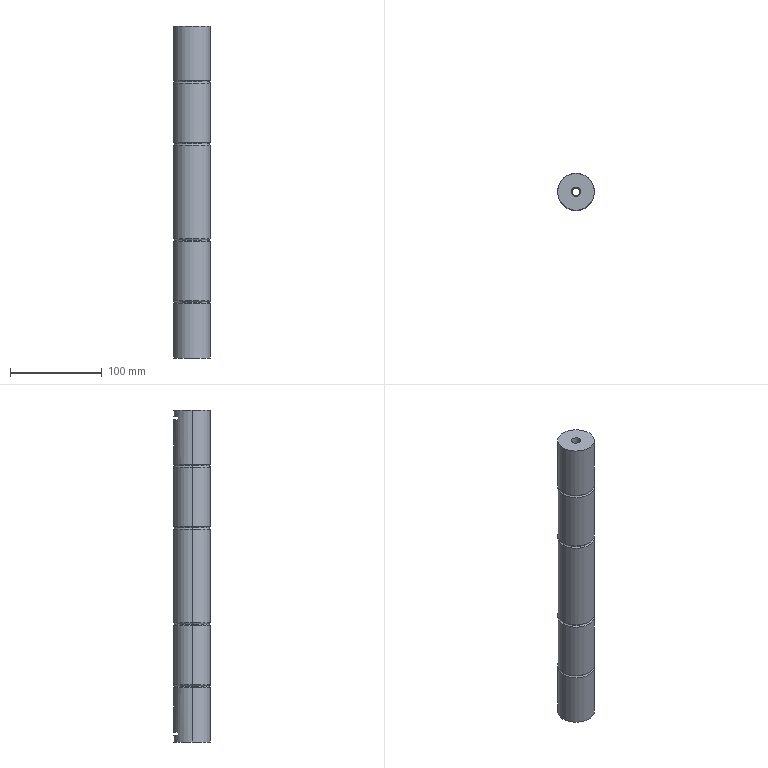Part | STEP file | LM-05-1232 | 1 solid | 58 faces | box 40 x 40 x 361 mm | volume 429924 mm3 | torus 24 | cylinder 20 | plane 10 | cone 4 | commonest cylinder face diameters 40 x10 3 x8 8.5 x2